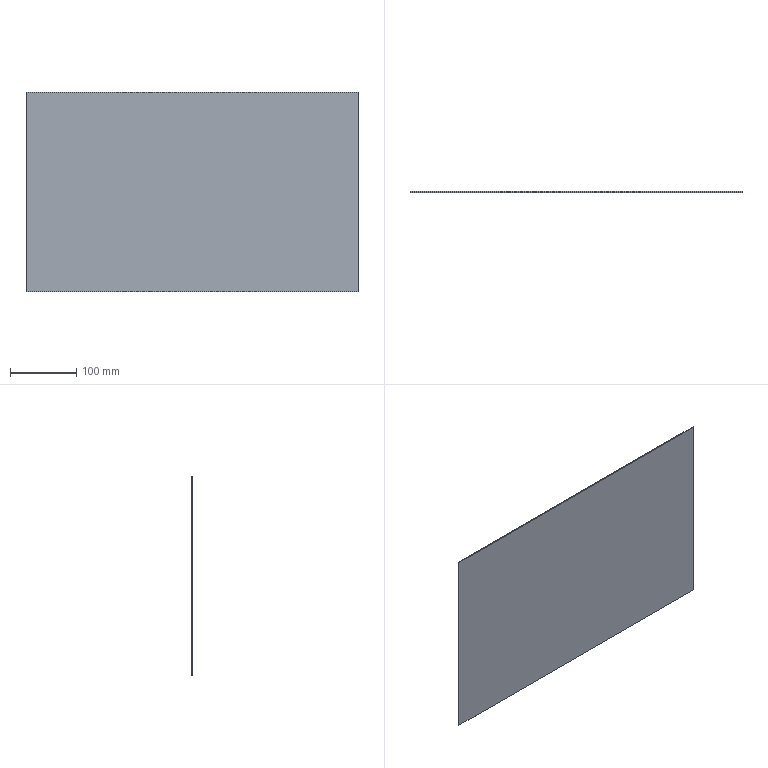Part | SolidWorks | features BaseBody 1 | 1 solid | 6 faces | box 500 x 1.5 x 300 mm | volume 225000 mm3 | plane 6
STEP:
#1=CARTESIAN_POINT('',(-250.,-1.5,-150.));
#2=VERTEX_POINT('',#1);
#3=CARTESIAN_POINT('',(250.,-1.5,-150.));
#4=VERTEX_POINT('',#3);
#5=CARTESIAN_POINT('',(-250.,-1.5,-150.));
#6=DIRECTION('',(1.,0.,0.));
#7=VECTOR('',#6,1000.);
#8=LINE('',#5,#7);
#9=EDGE_CURVE('',#2,#4,#8,.T.);
#10=ORIENTED_EDGE('',*,*,#9,.T.);
#11=CARTESIAN_POINT('',(250.,-1.5,150.));
#12=VERTEX_POINT('',#11);
#13=CARTESIAN_POINT('',(250.,-1.5,150.));
#14=DIRECTION('',(0.,0.,-1.));
#15=VECTOR('',#14,1000.);
#16=LINE('',#13,#15);
#17=EDGE_CURVE('',#12,#4,#16,.T.);
#18=ORIENTED_EDGE('',*,*,#17,.F.);
#19=CARTESIAN_POINT('',(-250.,-1.5,150.));
#20=VERTEX_POINT('',#19);
#21=CARTESIAN_POINT('',(-250.,-1.5,150.));
#22=DIRECTION('',(1.,0.,0.));
#23=VECTOR('',#22,1000.);
#24=LINE('',#21,#23);
#25=EDGE_CURVE('',#20,#12,#24,.T.);
#26=ORIENTED_EDGE('',*,*,#25,.F.);
#27=CARTESIAN_POINT('',(-250.,-1.5,150.));
#28=DIRECTION('',(0.,0.,-1.));
#29=VECTOR('',#28,1000.);
#30=LINE('',#27,#29);
#31=EDGE_CURVE('',#20,#2,#30,.T.);
#32=ORIENTED_EDGE('',*,*,#31,.T.);
#33=EDGE_LOOP('',(#10,#18,#26,#32));
#34=FACE_OUTER_BOUND('',#33,.T.);
#35=CARTESIAN_POINT('',(-250.,-1.5,150.));
#36=DIRECTION('',(0.,1.,0.));
#37=DIRECTION('',(-1.,0.,0.));
#38=AXIS2_PLACEMENT_3D('',#35,#36,#37);
#39=PLANE('',#38);
#40=ADVANCED_FACE('',(#34),#39,.F.);
#41=CARTESIAN_POINT('',(250.,0.,-150.));
#42=VERTEX_POINT('',#41);
#43=CARTESIAN_POINT('',(250.,0.,-150.));
#44=DIRECTION('',(0.,-1.,0.));
#45=VECTOR('',#44,1000.);
#46=LINE('',#43,#45);
#47=EDGE_CURVE('',#42,#4,#46,.T.);
#48=ORIENTED_EDGE('',*,*,#47,.F.);
#49=CARTESIAN_POINT('',(250.,0.,150.));
#50=VERTEX_POINT('',#49);
#51=CARTESIAN_POINT('',(250.,0.,150.));
#52=DIRECTION('',(0.,0.,-1.));
#53=VECTOR('',#52,1000.);
#54=LINE('',#51,#53);
#55=EDGE_CURVE('',#50,#42,#54,.T.);
#56=ORIENTED_EDGE('',*,*,#55,.F.);
#57=CARTESIAN_POINT('',(250.,0.,150.));
#58=DIRECTION('',(0.,-1.,0.));
#59=VECTOR('',#58,1000.);
#60=LINE('',#57,#59);
#61=EDGE_CURVE('',#50,#12,#60,.T.);
#62=ORIENTED_EDGE('',*,*,#61,.T.);
#63=ORIENTED_EDGE('',*,*,#17,.T.);
#64=EDGE_LOOP('',(#48,#56,#62,#63));
#65=FACE_OUTER_BOUND('',#64,.T.);
#66=CARTESIAN_POINT('',(250.,0.,150.));
#67=DIRECTION('',(1.,0.,0.));
#68=DIRECTION('',(0.,0.,-1.));
#69=AXIS2_PLACEMENT_3D('',#66,#67,#68);
#70=PLANE('',#69);
#71=ADVANCED_FACE('',(#65),#70,.T.);
#72=CARTESIAN_POINT('',(-250.,0.,-150.));
#73=VERTEX_POINT('',#72);
#74=CARTESIAN_POINT('',(-250.,0.,-150.));
#75=DIRECTION('',(1.,0.,0.));
#76=VECTOR('',#75,1000.);
#77=LINE('',#74,#76);
#78=EDGE_CURVE('',#73,#42,#77,.T.);
#79=ORIENTED_EDGE('',*,*,#78,.F.);
#80=CARTESIAN_POINT('',(-250.,0.,150.));
#81=VERTEX_POINT('',#80);
#82=CARTESIAN_POINT('',(-250.,0.,150.));
#83=DIRECTION('',(0.,0.,-1.));
#84=VECTOR('',#83,1000.);
#85=LINE('',#82,#84);
#86=EDGE_CURVE('',#81,#73,#85,.T.);
#87=ORIENTED_EDGE('',*,*,#86,.F.);
#88=CARTESIAN_POINT('',(-250.,0.,150.));
#89=DIRECTION('',(1.,0.,0.));
#90=VECTOR('',#89,1000.);
#91=LINE('',#88,#90);
#92=EDGE_CURVE('',#81,#50,#91,.T.);
#93=ORIENTED_EDGE('',*,*,#92,.T.);
#94=ORIENTED_EDGE('',*,*,#55,.T.);
#95=EDGE_LOOP('',(#79,#87,#93,#94));
#96=FACE_OUTER_BOUND('',#95,.T.);
#97=CARTESIAN_POINT('',(-250.,0.,150.));
#98=DIRECTION('',(0.,1.,0.));
#99=DIRECTION('',(-1.,0.,0.));
#100=AXIS2_PLACEMENT_3D('',#97,#98,#99);
#101=PLANE('',#100);
#102=ADVANCED_FACE('',(#96),#101,.T.);
#103=CARTESIAN_POINT('',(-250.,-1.5,-150.));
#104=DIRECTION('',(0.,1.,0.));
#105=VECTOR('',#104,1000.);
#106=LINE('',#103,#105);
#107=EDGE_CURVE('',#2,#73,#106,.T.);
#108=ORIENTED_EDGE('',*,*,#107,.F.);
#109=ORIENTED_EDGE('',*,*,#31,.F.);
#110=CARTESIAN_POINT('',(-250.,-1.5,150.));
#111=DIRECTION('',(0.,1.,0.));
#112=VECTOR('',#111,1000.);
#113=LINE('',#110,#112);
#114=EDGE_CURVE('',#20,#81,#113,.T.);
#115=ORIENTED_EDGE('',*,*,#114,.T.);
#116=ORIENTED_EDGE('',*,*,#86,.T.);
#117=EDGE_LOOP('',(#108,#109,#115,#116));
#118=FACE_OUTER_BOUND('',#117,.T.);
#119=CARTESIAN_POINT('',(-250.,-1.5,150.));
#120=DIRECTION('',(-1.,0.,0.));
#121=DIRECTION('',(0.,0.,1.));
#122=AXIS2_PLACEMENT_3D('',#119,#120,#121);
#123=PLANE('',#122);
#124=ADVANCED_FACE('',(#118),#123,.T.);
#125=ORIENTED_EDGE('',*,*,#25,.T.);
#126=ORIENTED_EDGE('',*,*,#61,.F.);
#127=ORIENTED_EDGE('',*,*,#92,.F.);
#128=ORIENTED_EDGE('',*,*,#114,.F.);
#129=EDGE_LOOP('',(#125,#126,#127,#128));
#130=FACE_OUTER_BOUND('',#129,.T.);
#131=CARTESIAN_POINT('',(0.,0.,150.));
#132=DIRECTION('',(0.,0.,-1.));
#133=DIRECTION('',(-1.,0.,0.));
#134=AXIS2_PLACEMENT_3D('',#131,#132,#133);
#135=PLANE('',#134);
#136=ADVANCED_FACE('',(#130),#135,.F.);
#137=ORIENTED_EDGE('',*,*,#9,.F.);
#138=ORIENTED_EDGE('',*,*,#107,.T.);
#139=ORIENTED_EDGE('',*,*,#78,.T.);
#140=ORIENTED_EDGE('',*,*,#47,.T.);
#141=EDGE_LOOP('',(#137,#138,#139,#140));
#142=FACE_OUTER_BOUND('',#141,.T.);
#143=CARTESIAN_POINT('',(0.,0.,-150.));
#144=DIRECTION('',(0.,0.,-1.));
#145=DIRECTION('',(-1.,0.,0.));
#146=AXIS2_PLACEMENT_3D('',#143,#144,#145);
#147=PLANE('',#146);
#148=ADVANCED_FACE('',(#142),#147,.T.);
#149=CLOSED_SHELL('',(#40,#71,#102,#124,#136,#148));
#150=MANIFOLD_SOLID_BREP('',#149);
#151=CARTESIAN_POINT('',(0.,0.,0.));
#152=DIRECTION('',(0.,0.,1.));
#153=DIRECTION('',(1.,0.,0.));
#154=AXIS2_PLACEMENT_3D('',#151,#152,#153);
#155=(LENGTH_UNIT()NAMED_UNIT(*)SI_UNIT(.MILLI.,.METRE.));
#156=UNCERTAINTY_MEASURE_WITH_UNIT(LENGTH_MEASURE(0.00001),#155,'','');
#157=(NAMED_UNIT(*)PLANE_ANGLE_UNIT()SI_UNIT($,.RADIAN.));
#158=(NAMED_UNIT(*)SI_UNIT($,.STERADIAN.)SOLID_ANGLE_UNIT());
#159=(GEOMETRIC_REPRESENTATION_CONTEXT(3)GLOBAL_UNCERTAINTY_ASSIGNED_CONTEXT((#156))GLOBAL_UNIT_ASSIGNED_CONTEXT((#155,#157,#158))REPRESENTATION_CONTEXT('',''));
#160=ADVANCED_BREP_SHAPE_REPRESENTATION('',(#150,#154),#159);